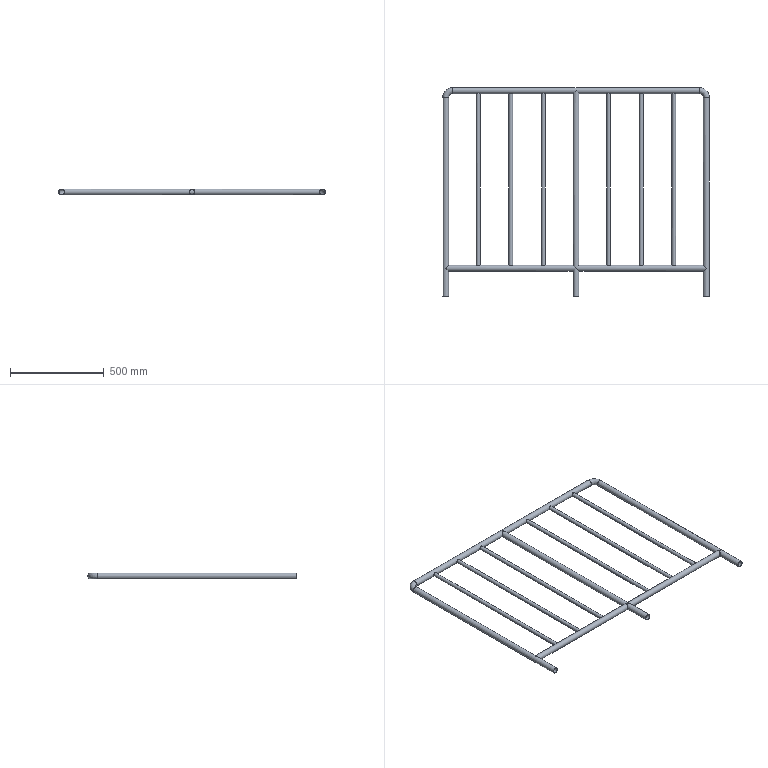Part | STEP file | 304 guardrail 1395X1100 body B_Default<As Machined> | 14 solids | 56 faces | box 1427 x 1116 x 32 mm | volume 1755808 mm3 | cylinder 41 | plane 11 | torus 4 | commonest cylinder face diameters 32 x23 16 x6 20 x6 28 x6